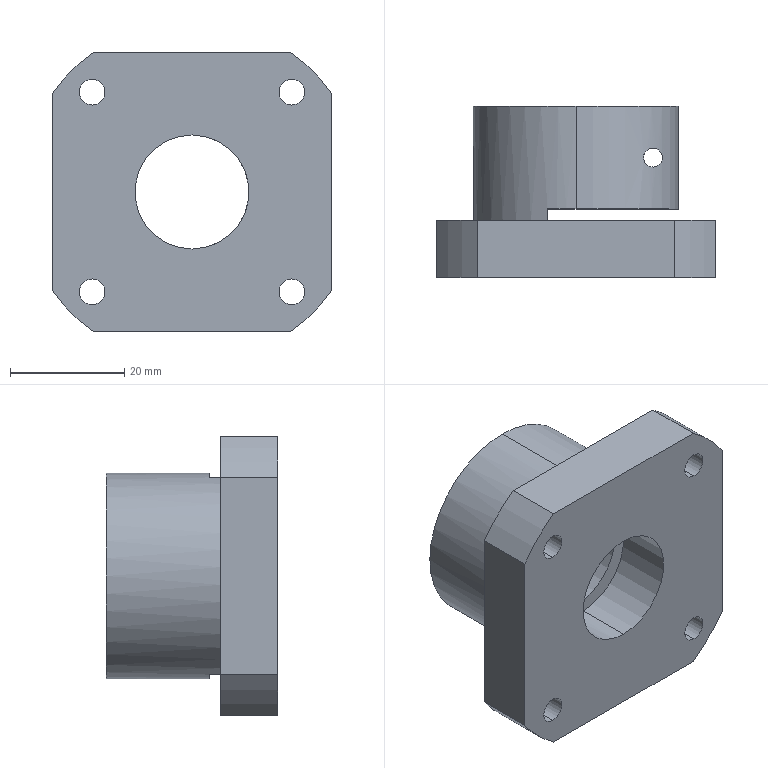Part | SolidWorks | features BaseBody 1 | 1 solid | 53 faces | box 49 x 30 x 49 mm | volume 31034 mm3 | cylinder 33 | plane 20 | commonest cylinder face diameters 4.5 x8 8 x8 20 x4 60 x4 36 x3 3.3 x2